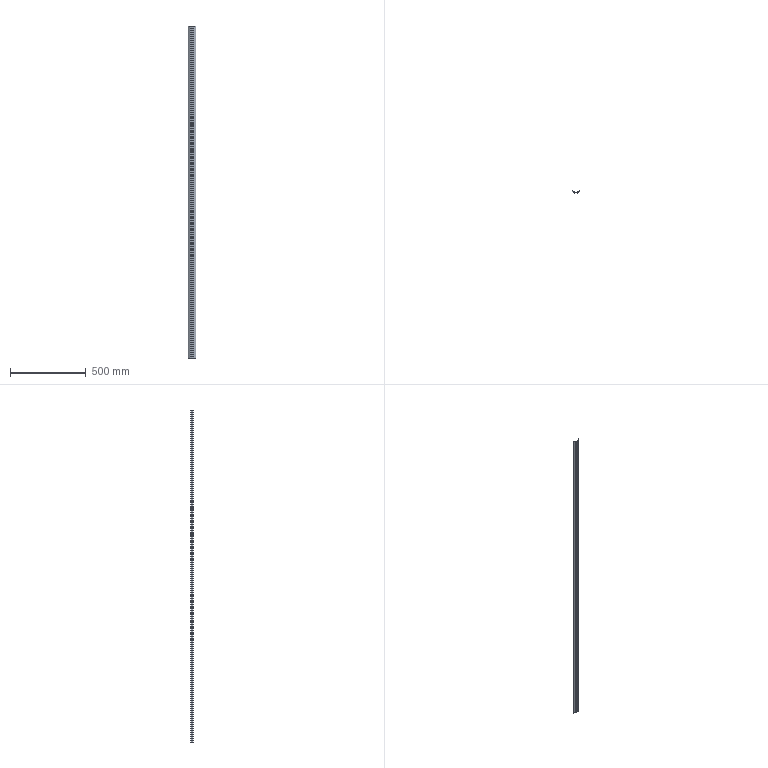Part | 1 solid | 32 faces | box 46.782 x 13.535 x 2190 mm | volume 175881 mm3 | plane 25 | cylinder 7 | commonest cylinder face diameters 67.994 x4 0.2 x2 65.594 x1
STEP:
#1=CARTESIAN_POINT('',(-11.25,9.786,-1095.));
#2=VERTEX_POINT('',#1);
#3=CARTESIAN_POINT('',(-11.25,5.783,-1095.));
#4=VERTEX_POINT('',#3);
#5=CARTESIAN_POINT('',(-11.25,9.786,-1095.));
#6=DIRECTION('',(0.,-1.,0.));
#7=VECTOR('',#6,1000.);
#8=LINE('',#5,#7);
#9=EDGE_CURVE('',#2,#4,#8,.T.);
#10=ORIENTED_EDGE('',*,*,#9,.T.);
#11=CARTESIAN_POINT('',(-11.25,5.783,1095.));
#12=VERTEX_POINT('',#11);
#13=CARTESIAN_POINT('',(-11.25,5.783,1095.));
#14=DIRECTION('',(0.,0.,-1.));
#15=VECTOR('',#14,1000.);
#16=LINE('',#13,#15);
#17=EDGE_CURVE('',#12,#4,#16,.T.);
#18=ORIENTED_EDGE('',*,*,#17,.F.);
#19=CARTESIAN_POINT('',(-11.25,9.786,1095.));
#20=VERTEX_POINT('',#19);
#21=CARTESIAN_POINT('',(-11.25,9.786,1095.));
#22=DIRECTION('',(0.,-1.,0.));
#23=VECTOR('',#22,1000.);
#24=LINE('',#21,#23);
#25=EDGE_CURVE('',#20,#12,#24,.T.);
#26=ORIENTED_EDGE('',*,*,#25,.F.);
#27=CARTESIAN_POINT('',(-11.25,9.786,1095.));
#28=DIRECTION('',(0.,0.,-1.));
#29=VECTOR('',#28,1000.);
#30=LINE('',#27,#29);
#31=EDGE_CURVE('',#20,#2,#30,.T.);
#32=ORIENTED_EDGE('',*,*,#31,.T.);
#33=EDGE_LOOP('',(#10,#18,#26,#32));
#34=FACE_OUTER_BOUND('',#33,.T.);
#35=CARTESIAN_POINT('',(-11.25,9.786,1095.));
#36=DIRECTION('',(1.,0.,0.));
#37=DIRECTION('',(0.,0.,-1.));
#38=AXIS2_PLACEMENT_3D('',#35,#36,#37);
#39=PLANE('',#38);
#40=ADVANCED_FACE('',(#34),#39,.F.);
#41=CARTESIAN_POINT('',(-10.667,5.2,-1095.));
#42=VERTEX_POINT('',#41);
#43=CARTESIAN_POINT('',(-11.25,5.783,-1095.));
#44=DIRECTION('',(0.7071,-0.7071,0.));
#45=VECTOR('',#44,1000.);
#46=LINE('',#43,#45);
#47=EDGE_CURVE('',#4,#42,#46,.T.);
#48=ORIENTED_EDGE('',*,*,#47,.T.);
#49=CARTESIAN_POINT('',(-10.667,5.2,1095.));
#50=VERTEX_POINT('',#49);
#51=CARTESIAN_POINT('',(-10.667,5.2,1095.));
#52=DIRECTION('',(0.,0.,-1.));
#53=VECTOR('',#52,1000.);
#54=LINE('',#51,#53);
#55=EDGE_CURVE('',#50,#42,#54,.T.);
#56=ORIENTED_EDGE('',*,*,#55,.F.);
#57=CARTESIAN_POINT('',(-11.25,5.783,1095.));
#58=DIRECTION('',(0.7071,-0.7071,0.));
#59=VECTOR('',#58,1000.);
#60=LINE('',#57,#59);
#61=EDGE_CURVE('',#12,#50,#60,.T.);
#62=ORIENTED_EDGE('',*,*,#61,.F.);
#63=ORIENTED_EDGE('',*,*,#17,.T.);
#64=EDGE_LOOP('',(#48,#56,#62,#63));
#65=FACE_OUTER_BOUND('',#64,.T.);
#66=CARTESIAN_POINT('',(-11.25,5.783,1095.));
#67=DIRECTION('',(0.7071,0.7071,0.));
#68=DIRECTION('',(-0.7071,0.7071,0.));
#69=AXIS2_PLACEMENT_3D('',#66,#67,#68);
#70=PLANE('',#69);
#71=ADVANCED_FACE('',(#65),#70,.F.);
#72=CARTESIAN_POINT('',(-8.25,5.2,-1095.));
#73=VERTEX_POINT('',#72);
#74=CARTESIAN_POINT('',(-10.667,5.2,-1095.));
#75=DIRECTION('',(1.,0.,0.));
#76=VECTOR('',#75,1000.);
#77=LINE('',#74,#76);
#78=EDGE_CURVE('',#42,#73,#77,.T.);
#79=ORIENTED_EDGE('',*,*,#78,.T.);
#80=CARTESIAN_POINT('',(-8.25,5.2,1095.));
#81=VERTEX_POINT('',#80);
#82=CARTESIAN_POINT('',(-8.25,5.2,1095.));
#83=DIRECTION('',(0.,0.,-1.));
#84=VECTOR('',#83,1000.);
#85=LINE('',#82,#84);
#86=EDGE_CURVE('',#81,#73,#85,.T.);
#87=ORIENTED_EDGE('',*,*,#86,.F.);
#88=CARTESIAN_POINT('',(-10.667,5.2,1095.));
#89=DIRECTION('',(1.,0.,0.));
#90=VECTOR('',#89,1000.);
#91=LINE('',#88,#90);
#92=EDGE_CURVE('',#50,#81,#91,.T.);
#93=ORIENTED_EDGE('',*,*,#92,.F.);
#94=ORIENTED_EDGE('',*,*,#55,.T.);
#95=EDGE_LOOP('',(#79,#87,#93,#94));
#96=FACE_OUTER_BOUND('',#95,.T.);
#97=CARTESIAN_POINT('',(-10.667,5.2,1095.));
#98=DIRECTION('',(0.,1.,0.));
#99=DIRECTION('',(0.,0.,1.));
#100=AXIS2_PLACEMENT_3D('',#97,#98,#99);
#101=PLANE('',#100);
#102=ADVANCED_FACE('',(#96),#101,.F.);
#103=CARTESIAN_POINT('',(-8.25,6.,-1095.));
#104=VERTEX_POINT('',#103);
#105=CARTESIAN_POINT('',(-8.25,5.2,-1095.));
#106=DIRECTION('',(0.,1.,0.));
#107=VECTOR('',#106,1000.);
#108=LINE('',#105,#107);
#109=EDGE_CURVE('',#73,#104,#108,.T.);
#110=ORIENTED_EDGE('',*,*,#109,.T.);
#111=CARTESIAN_POINT('',(-8.25,6.,1095.));
#112=VERTEX_POINT('',#111);
#113=CARTESIAN_POINT('',(-8.25,6.,1095.));
#114=DIRECTION('',(0.,0.,-1.));
#115=VECTOR('',#114,1000.);
#116=LINE('',#113,#115);
#117=EDGE_CURVE('',#112,#104,#116,.T.);
#118=ORIENTED_EDGE('',*,*,#117,.F.);
#119=CARTESIAN_POINT('',(-8.25,5.2,1095.));
#120=DIRECTION('',(0.,1.,0.));
#121=VECTOR('',#120,1000.);
#122=LINE('',#119,#121);
#123=EDGE_CURVE('',#81,#112,#122,.T.);
#124=ORIENTED_EDGE('',*,*,#123,.F.);
#125=ORIENTED_EDGE('',*,*,#86,.T.);
#126=EDGE_LOOP('',(#110,#118,#124,#125));
#127=FACE_OUTER_BOUND('',#126,.T.);
#128=CARTESIAN_POINT('',(-8.25,5.2,1095.));
#129=DIRECTION('',(-1.,0.,0.));
#130=DIRECTION('',(0.,0.,1.));
#131=AXIS2_PLACEMENT_3D('',#128,#129,#130);
#132=PLANE('',#131);
#133=ADVANCED_FACE('',(#127),#132,.F.);
#134=CARTESIAN_POINT('',(-10.25,6.,-1095.));
#135=VERTEX_POINT('',#134);
#136=CARTESIAN_POINT('',(-8.25,6.,-1095.));
#137=DIRECTION('',(-1.,0.,0.));
#138=VECTOR('',#137,1000.);
#139=LINE('',#136,#138);
#140=EDGE_CURVE('',#104,#135,#139,.T.);
#141=ORIENTED_EDGE('',*,*,#140,.T.);
#142=CARTESIAN_POINT('',(-10.25,6.,1095.));
#143=VERTEX_POINT('',#142);
#144=CARTESIAN_POINT('',(-10.25,6.,1095.));
#145=DIRECTION('',(0.,0.,-1.));
#146=VECTOR('',#145,1000.);
#147=LINE('',#144,#146);
#148=EDGE_CURVE('',#143,#135,#147,.T.);
#149=ORIENTED_EDGE('',*,*,#148,.F.);
#150=CARTESIAN_POINT('',(-8.25,6.,1095.));
#151=DIRECTION('',(-1.,0.,0.));
#152=VECTOR('',#151,1000.);
#153=LINE('',#150,#152);
#154=EDGE_CURVE('',#112,#143,#153,.T.);
#155=ORIENTED_EDGE('',*,*,#154,.F.);
#156=ORIENTED_EDGE('',*,*,#117,.T.);
#157=EDGE_LOOP('',(#141,#149,#155,#156));
#158=FACE_OUTER_BOUND('',#157,.T.);
#159=CARTESIAN_POINT('',(-8.25,6.,1095.));
#160=DIRECTION('',(0.,-1.,0.));
#161=DIRECTION('',(0.,0.,-1.));
#162=AXIS2_PLACEMENT_3D('',#159,#160,#161);
#163=PLANE('',#162);
#164=ADVANCED_FACE('',(#158),#163,.F.);
#165=CARTESIAN_POINT('',(-10.25,7.726,-1095.));
#166=VERTEX_POINT('',#165);
#167=CARTESIAN_POINT('',(-10.25,6.,-1095.));
#168=DIRECTION('',(0.,1.,0.));
#169=VECTOR('',#168,1000.);
#170=LINE('',#167,#169);
#171=EDGE_CURVE('',#135,#166,#170,.T.);
#172=ORIENTED_EDGE('',*,*,#171,.T.);
#173=CARTESIAN_POINT('',(-10.25,7.726,1095.));
#174=VERTEX_POINT('',#173);
#175=CARTESIAN_POINT('',(-10.25,7.726,1095.));
#176=DIRECTION('',(0.,0.,-1.));
#177=VECTOR('',#176,1000.);
#178=LINE('',#175,#177);
#179=EDGE_CURVE('',#174,#166,#178,.T.);
#180=ORIENTED_EDGE('',*,*,#179,.F.);
#181=CARTESIAN_POINT('',(-10.25,6.,1095.));
#182=DIRECTION('',(0.,1.,0.));
#183=VECTOR('',#182,1000.);
#184=LINE('',#181,#183);
#185=EDGE_CURVE('',#143,#174,#184,.T.);
#186=ORIENTED_EDGE('',*,*,#185,.F.);
#187=ORIENTED_EDGE('',*,*,#148,.T.);
#188=EDGE_LOOP('',(#172,#180,#186,#187));
#189=FACE_OUTER_BOUND('',#188,.T.);
#190=CARTESIAN_POINT('',(-10.25,6.,1095.));
#191=DIRECTION('',(-1.,0.,0.));
#192=DIRECTION('',(0.,0.,1.));
#193=AXIS2_PLACEMENT_3D('',#190,#191,#192);
#194=PLANE('',#193);
#195=ADVANCED_FACE('',(#189),#194,.F.);
#196=CARTESIAN_POINT('',(-9.,7.725,-1095.));
#197=VERTEX_POINT('',#196);
#198=CARTESIAN_POINT('',(-10.25,7.726,-1095.));
#199=DIRECTION('',(1.,-0.001291,0.));
#200=VECTOR('',#199,1000.);
#201=LINE('',#198,#200);
#202=EDGE_CURVE('',#166,#197,#201,.T.);
#203=ORIENTED_EDGE('',*,*,#202,.T.);
#204=CARTESIAN_POINT('',(-9.,7.725,1095.));
#205=VERTEX_POINT('',#204);
#206=CARTESIAN_POINT('',(-9.,7.725,1095.));
#207=DIRECTION('',(0.,0.,-1.));
#208=VECTOR('',#207,1000.);
#209=LINE('',#206,#208);
#210=EDGE_CURVE('',#205,#197,#209,.T.);
#211=ORIENTED_EDGE('',*,*,#210,.F.);
#212=CARTESIAN_POINT('',(-10.25,7.726,1095.));
#213=DIRECTION('',(1.,-0.001291,0.));
#214=VECTOR('',#213,1000.);
#215=LINE('',#212,#214);
#216=EDGE_CURVE('',#174,#205,#215,.T.);
#217=ORIENTED_EDGE('',*,*,#216,.F.);
#218=ORIENTED_EDGE('',*,*,#179,.T.);
#219=EDGE_LOOP('',(#203,#211,#217,#218));
#220=FACE_OUTER_BOUND('',#219,.T.);
#221=CARTESIAN_POINT('',(-10.25,7.726,1095.));
#222=DIRECTION('',(0.001291,1.,0.));
#223=DIRECTION('',(-1.,0.001291,0.));
#224=AXIS2_PLACEMENT_3D('',#221,#222,#223);
#225=PLANE('',#224);
#226=ADVANCED_FACE('',(#220),#225,.F.);
#227=CARTESIAN_POINT('',(-8.25,8.474,-1095.));
#228=VERTEX_POINT('',#227);
#229=CARTESIAN_POINT('',(-9.,7.725,-1095.));
#230=DIRECTION('',(0.7076,0.7067,0.));
#231=VECTOR('',#230,1000.);
#232=LINE('',#229,#231);
#233=EDGE_CURVE('',#197,#228,#232,.T.);
#234=ORIENTED_EDGE('',*,*,#233,.T.);
#235=CARTESIAN_POINT('',(-8.25,8.474,1095.));
#236=VERTEX_POINT('',#235);
#237=CARTESIAN_POINT('',(-8.25,8.474,1095.));
#238=DIRECTION('',(0.,0.,-1.));
#239=VECTOR('',#238,1000.);
#240=LINE('',#237,#239);
#241=EDGE_CURVE('',#236,#228,#240,.T.);
#242=ORIENTED_EDGE('',*,*,#241,.F.);
#243=CARTESIAN_POINT('',(-9.,7.725,1095.));
#244=DIRECTION('',(0.7076,0.7067,0.));
#245=VECTOR('',#244,1000.);
#246=LINE('',#243,#245);
#247=EDGE_CURVE('',#205,#236,#246,.T.);
#248=ORIENTED_EDGE('',*,*,#247,.F.);
#249=ORIENTED_EDGE('',*,*,#210,.T.);
#250=EDGE_LOOP('',(#234,#242,#248,#249));
#251=FACE_OUTER_BOUND('',#250,.T.);
#252=CARTESIAN_POINT('',(-9.,7.725,1095.));
#253=DIRECTION('',(-0.7067,0.7076,0.));
#254=DIRECTION('',(-0.7076,-0.7067,0.));
#255=AXIS2_PLACEMENT_3D('',#252,#253,#254);
#256=PLANE('',#255);
#257=ADVANCED_FACE('',(#251),#256,.F.);
#258=CARTESIAN_POINT('',(-8.25,8.887,-1095.));
#259=VERTEX_POINT('',#258);
#260=CARTESIAN_POINT('',(-8.25,8.474,-1095.));
#261=DIRECTION('',(0.,1.,0.));
#262=VECTOR('',#261,1000.);
#263=LINE('',#260,#262);
#264=EDGE_CURVE('',#228,#259,#263,.T.);
#265=ORIENTED_EDGE('',*,*,#264,.T.);
#266=CARTESIAN_POINT('',(-8.25,8.887,1095.));
#267=VERTEX_POINT('',#266);
#268=CARTESIAN_POINT('',(-8.25,8.887,1095.));
#269=DIRECTION('',(0.,0.,-1.));
#270=VECTOR('',#269,1000.);
#271=LINE('',#268,#270);
#272=EDGE_CURVE('',#267,#259,#271,.T.);
#273=ORIENTED_EDGE('',*,*,#272,.F.);
#274=CARTESIAN_POINT('',(-8.25,8.474,1095.));
#275=DIRECTION('',(0.,1.,0.));
#276=VECTOR('',#275,1000.);
#277=LINE('',#274,#276);
#278=EDGE_CURVE('',#236,#267,#277,.T.);
#279=ORIENTED_EDGE('',*,*,#278,.F.);
#280=ORIENTED_EDGE('',*,*,#241,.T.);
#281=EDGE_LOOP('',(#265,#273,#279,#280));
#282=FACE_OUTER_BOUND('',#281,.T.);
#283=CARTESIAN_POINT('',(-8.25,8.474,1095.));
#284=DIRECTION('',(-1.,0.,0.));
#285=DIRECTION('',(0.,0.,1.));
#286=AXIS2_PLACEMENT_3D('',#283,#284,#285);
#287=PLANE('',#286);
#288=ADVANCED_FACE('',(#282),#287,.F.);
#289=CARTESIAN_POINT('',(-3.,8.003,-1095.));
#290=VERTEX_POINT('',#289);
#291=CARTESIAN_POINT('',(0.,41.867,-1095.));
#292=DIRECTION('',(0.,0.,1.));
#293=DIRECTION('',(1.,0.,0.));
#294=AXIS2_PLACEMENT_3D('',#291,#292,#293);
#295=CIRCLE('',#294,33.997);
#296=EDGE_CURVE('',#259,#290,#295,.T.);
#297=ORIENTED_EDGE('',*,*,#296,.T.);
#298=CARTESIAN_POINT('',(-3.,8.003,1095.));
#299=VERTEX_POINT('',#298);
#300=CARTESIAN_POINT('',(-3.,8.003,1095.));
#301=DIRECTION('',(0.,0.,-1.));
#302=VECTOR('',#301,1000.);
#303=LINE('',#300,#302);
#304=EDGE_CURVE('',#299,#290,#303,.T.);
#305=ORIENTED_EDGE('',*,*,#304,.F.);
#306=CARTESIAN_POINT('',(0.,41.867,1095.));
#307=DIRECTION('',(0.,0.,1.));
#308=DIRECTION('',(1.,0.,0.));
#309=AXIS2_PLACEMENT_3D('',#306,#307,#308);
#310=CIRCLE('',#309,33.997);
#311=EDGE_CURVE('',#267,#299,#310,.T.);
#312=ORIENTED_EDGE('',*,*,#311,.F.);
#313=ORIENTED_EDGE('',*,*,#272,.T.);
#314=EDGE_LOOP('',(#297,#305,#312,#313));
#315=FACE_OUTER_BOUND('',#314,.T.);
#316=CARTESIAN_POINT('',(0.,41.867,1095.));
#317=DIRECTION('',(0.,0.,-1.));
#318=DIRECTION('',(-1.,0.,0.));
#319=AXIS2_PLACEMENT_3D('',#316,#317,#318);
#320=CYLINDRICAL_SURFACE('',#319,33.997);
#321=ADVANCED_FACE('',(#315),#320,.T.);
#322=CARTESIAN_POINT('',(-3.,7.702,-1095.));
#323=VERTEX_POINT('',#322);
#324=CARTESIAN_POINT('',(-3.,8.003,-1095.));
#325=DIRECTION('',(0.,-1.,0.));
#326=VECTOR('',#325,1000.);
#327=LINE('',#324,#326);
#328=EDGE_CURVE('',#290,#323,#327,.T.);
#329=ORIENTED_EDGE('',*,*,#328,.T.);
#330=CARTESIAN_POINT('',(-3.,7.702,1095.));
#331=VERTEX_POINT('',#330);
#332=CARTESIAN_POINT('',(-3.,7.702,1095.));
#333=DIRECTION('',(0.,0.,-1.));
#334=VECTOR('',#333,1000.);
#335=LINE('',#332,#334);
#336=EDGE_CURVE('',#331,#323,#335,.T.);
#337=ORIENTED_EDGE('',*,*,#336,.F.);
#338=CARTESIAN_POINT('',(-3.,8.003,1095.));
#339=DIRECTION('',(0.,-1.,0.));
#340=VECTOR('',#339,1000.);
#341=LINE('',#338,#340);
#342=EDGE_CURVE('',#299,#331,#341,.T.);
#343=ORIENTED_EDGE('',*,*,#342,.F.);
#344=ORIENTED_EDGE('',*,*,#304,.T.);
#345=EDGE_LOOP('',(#329,#337,#343,#344));
#346=FACE_OUTER_BOUND('',#345,.T.);
#347=CARTESIAN_POINT('',(-3.,8.003,1095.));
#348=DIRECTION('',(1.,0.,0.));
#349=DIRECTION('',(0.,0.,-1.));
#350=AXIS2_PLACEMENT_3D('',#347,#348,#349);
#351=PLANE('',#350);
#352=ADVANCED_FACE('',(#346),#351,.F.);
#353=CARTESIAN_POINT('',(3.,7.702,-1095.));
#354=VERTEX_POINT('',#353);
#355=CARTESIAN_POINT('',(-3.,7.702,-1095.));
#356=DIRECTION('',(1.,0.,0.));
#357=VECTOR('',#356,1000.);
#358=LINE('',#355,#357);
#359=EDGE_CURVE('',#323,#354,#358,.T.);
#360=ORIENTED_EDGE('',*,*,#359,.T.);
#361=CARTESIAN_POINT('',(3.,7.702,1095.));
#362=VERTEX_POINT('',#361);
#363=CARTESIAN_POINT('',(3.,7.702,1095.));
#364=DIRECTION('',(0.,0.,-1.));
#365=VECTOR('',#364,1000.);
#366=LINE('',#363,#365);
#367=EDGE_CURVE('',#362,#354,#366,.T.);
#368=ORIENTED_EDGE('',*,*,#367,.F.);
#369=CARTESIAN_POINT('',(-3.,7.702,1095.));
#370=DIRECTION('',(1.,0.,0.));
#371=VECTOR('',#370,1000.);
#372=LINE('',#369,#371);
#373=EDGE_CURVE('',#331,#362,#372,.T.);
#374=ORIENTED_EDGE('',*,*,#373,.F.);
#375=ORIENTED_EDGE('',*,*,#336,.T.);
#376=EDGE_LOOP('',(#360,#368,#374,#375));
#377=FACE_OUTER_BOUND('',#376,.T.);
#378=CARTESIAN_POINT('',(-3.,7.702,1095.));
#379=DIRECTION('',(0.,1.,0.));
#380=DIRECTION('',(0.,0.,1.));
#381=AXIS2_PLACEMENT_3D('',#378,#379,#380);
#382=PLANE('',#381);
#383=ADVANCED_FACE('',(#377),#382,.F.);
#384=CARTESIAN_POINT('',(3.,8.003,-1095.));
#385=VERTEX_POINT('',#384);
#386=CARTESIAN_POINT('',(3.,7.702,-1095.));
#387=DIRECTION('',(0.,1.,0.));
#388=VECTOR('',#387,1000.);
#389=LINE('',#386,#388);
#390=EDGE_CURVE('',#354,#385,#389,.T.);
#391=ORIENTED_EDGE('',*,*,#390,.T.);
#392=CARTESIAN_POINT('',(3.,8.003,1095.));
#393=VERTEX_POINT('',#392);
#394=CARTESIAN_POINT('',(3.,8.003,1095.));
#395=DIRECTION('',(0.,0.,-1.));
#396=VECTOR('',#395,1000.);
#397=LINE('',#394,#396);
#398=EDGE_CURVE('',#393,#385,#397,.T.);
#399=ORIENTED_EDGE('',*,*,#398,.F.);
#400=CARTESIAN_POINT('',(3.,7.702,1095.));
#401=DIRECTION('',(0.,1.,0.));
#402=VECTOR('',#401,1000.);
#403=LINE('',#400,#402);
#404=EDGE_CURVE('',#362,#393,#403,.T.);
#405=ORIENTED_EDGE('',*,*,#404,.F.);
#406=ORIENTED_EDGE('',*,*,#367,.T.);
#407=EDGE_LOOP('',(#391,#399,#405,#406));
#408=FACE_OUTER_BOUND('',#407,.T.);
#409=CARTESIAN_POINT('',(3.,7.702,1095.));
#410=DIRECTION('',(-1.,0.,0.));
#411=DIRECTION('',(0.,0.,1.));
#412=AXIS2_PLACEMENT_3D('',#409,#410,#411);
#413=PLANE('',#412);
#414=ADVANCED_FACE('',(#408),#413,.F.);
#415=CARTESIAN_POINT('',(8.25,8.887,-1095.));
#416=VERTEX_POINT('',#415);
#417=CARTESIAN_POINT('',(0.,41.867,-1095.));
#418=DIRECTION('',(0.,0.,1.));
#419=DIRECTION('',(1.,0.,0.));
#420=AXIS2_PLACEMENT_3D('',#417,#418,#419);
#421=CIRCLE('',#420,33.997);
#422=EDGE_CURVE('',#385,#416,#421,.T.);
#423=ORIENTED_EDGE('',*,*,#422,.T.);
#424=CARTESIAN_POINT('',(8.25,8.887,1095.));
#425=VERTEX_POINT('',#424);
#426=CARTESIAN_POINT('',(8.25,8.887,1095.));
#427=DIRECTION('',(0.,0.,-1.));
#428=VECTOR('',#427,1000.);
#429=LINE('',#426,#428);
#430=EDGE_CURVE('',#425,#416,#429,.T.);
#431=ORIENTED_EDGE('',*,*,#430,.F.);
#432=CARTESIAN_POINT('',(0.,41.867,1095.));
#433=DIRECTION('',(0.,0.,1.));
#434=DIRECTION('',(1.,0.,0.));
#435=AXIS2_PLACEMENT_3D('',#432,#433,#434);
#436=CIRCLE('',#435,33.997);
#437=EDGE_CURVE('',#393,#425,#436,.T.);
#438=ORIENTED_EDGE('',*,*,#437,.F.);
#439=ORIENTED_EDGE('',*,*,#398,.T.);
#440=EDGE_LOOP('',(#423,#431,#438,#439));
#441=FACE_OUTER_BOUND('',#440,.T.);
#442=CARTESIAN_POINT('',(0.,41.867,1095.));
#443=DIRECTION('',(0.,0.,-1.));
#444=DIRECTION('',(-1.,0.,0.));
#445=AXIS2_PLACEMENT_3D('',#442,#443,#444);
#446=CYLINDRICAL_SURFACE('',#445,33.997);
#447=ADVANCED_FACE('',(#441),#446,.T.);
#448=CARTESIAN_POINT('',(8.25,8.474,-1095.));
#449=VERTEX_POINT('',#448);
#450=CARTESIAN_POINT('',(8.25,8.887,-1095.));
#451=DIRECTION('',(0.,-1.,0.));
#452=VECTOR('',#451,1000.);
#453=LINE('',#450,#452);
#454=EDGE_CURVE('',#416,#449,#453,.T.);
#455=ORIENTED_EDGE('',*,*,#454,.T.);
#456=CARTESIAN_POINT('',(8.25,8.474,1095.));
#457=VERTEX_POINT('',#456);
#458=CARTESIAN_POINT('',(8.25,8.474,1095.));
#459=DIRECTION('',(0.,0.,-1.));
#460=VECTOR('',#459,1000.);
#461=LINE('',#458,#460);
#462=EDGE_CURVE('',#457,#449,#461,.T.);
#463=ORIENTED_EDGE('',*,*,#462,.F.);
#464=CARTESIAN_POINT('',(8.25,8.887,1095.));
#465=DIRECTION('',(0.,-1.,0.));
#466=VECTOR('',#465,1000.);
#467=LINE('',#464,#466);
#468=EDGE_CURVE('',#425,#457,#467,.T.);
#469=ORIENTED_EDGE('',*,*,#468,.F.);
#470=ORIENTED_EDGE('',*,*,#430,.T.);
#471=EDGE_LOOP('',(#455,#463,#469,#470));
#472=FACE_OUTER_BOUND('',#471,.T.);
#473=CARTESIAN_POINT('',(8.25,8.887,1095.));
#474=DIRECTION('',(1.,0.,0.));
#475=DIRECTION('',(0.,0.,-1.));
#476=AXIS2_PLACEMENT_3D('',#473,#474,#475);
#477=PLANE('',#476);
#478=ADVANCED_FACE('',(#472),#477,.F.);
#479=CARTESIAN_POINT('',(9.,7.725,-1095.));
#480=VERTEX_POINT('',#479);
#481=CARTESIAN_POINT('',(8.25,8.474,-1095.));
#482=DIRECTION('',(0.7076,-0.7067,0.));
#483=VECTOR('',#482,1000.);
#484=LINE('',#481,#483);
#485=EDGE_CURVE('',#449,#480,#484,.T.);
#486=ORIENTED_EDGE('',*,*,#485,.T.);
#487=CARTESIAN_POINT('',(9.,7.725,1095.));
#488=VERTEX_POINT('',#487);
#489=CARTESIAN_POINT('',(9.,7.725,1095.));
#490=DIRECTION('',(0.,0.,-1.));
#491=VECTOR('',#490,1000.);
#492=LINE('',#489,#491);
#493=EDGE_CURVE('',#488,#480,#492,.T.);
#494=ORIENTED_EDGE('',*,*,#493,.F.);
#495=CARTESIAN_POINT('',(8.25,8.474,1095.));
#496=DIRECTION('',(0.7076,-0.7067,0.));
#497=VECTOR('',#496,1000.);
#498=LINE('',#495,#497);
#499=EDGE_CURVE('',#457,#488,#498,.T.);
#500=ORIENTED_EDGE('',*,*,#499,.F.);
#501=ORIENTED_EDGE('',*,*,#462,.T.);
#502=EDGE_LOOP('',(#486,#494,#500,#501));
#503=FACE_OUTER_BOUND('',#502,.T.);
#504=CARTESIAN_POINT('',(8.25,8.474,1095.));
#505=DIRECTION('',(0.7067,0.7076,0.));
#506=DIRECTION('',(-0.7076,0.7067,0.));
#507=AXIS2_PLACEMENT_3D('',#504,#505,#506);
#508=PLANE('',#507);
#509=ADVANCED_FACE('',(#503),#508,.F.);
#510=CARTESIAN_POINT('',(10.25,7.726,-1095.));
#511=VERTEX_POINT('',#510);
#512=CARTESIAN_POINT('',(9.,7.725,-1095.));
#513=DIRECTION('',(1.,0.001291,0.));
#514=VECTOR('',#513,1000.);
#515=LINE('',#512,#514);
#516=EDGE_CURVE('',#480,#511,#515,.T.);
#517=ORIENTED_EDGE('',*,*,#516,.T.);
#518=CARTESIAN_POINT('',(10.25,7.726,1095.));
#519=VERTEX_POINT('',#518);
#520=CARTESIAN_POINT('',(10.25,7.726,1095.));
#521=DIRECTION('',(0.,0.,-1.));
#522=VECTOR('',#521,1000.);
#523=LINE('',#520,#522);
#524=EDGE_CURVE('',#519,#511,#523,.T.);
#525=ORIENTED_EDGE('',*,*,#524,.F.);
#526=CARTESIAN_POINT('',(9.,7.725,1095.));
#527=DIRECTION('',(1.,0.001291,0.));
#528=VECTOR('',#527,1000.);
#529=LINE('',#526,#528);
#530=EDGE_CURVE('',#488,#519,#529,.T.);
#531=ORIENTED_EDGE('',*,*,#530,.F.);
#532=ORIENTED_EDGE('',*,*,#493,.T.);
#533=EDGE_LOOP('',(#517,#525,#531,#532));
#534=FACE_OUTER_BOUND('',#533,.T.);
#535=CARTESIAN_POINT('',(9.,7.725,1095.));
#536=DIRECTION('',(-0.001291,1.,0.));
#537=DIRECTION('',(-1.,-0.001291,0.));
#538=AXIS2_PLACEMENT_3D('',#535,#536,#537);
#539=PLANE('',#538);
#540=ADVANCED_FACE('',(#534),#539,.F.);
#541=CARTESIAN_POINT('',(10.25,6.,-1095.));
#542=VERTEX_POINT('',#541);
#543=CARTESIAN_POINT('',(10.25,7.726,-1095.));
#544=DIRECTION('',(0.,-1.,0.));
#545=VECTOR('',#544,1000.);
#546=LINE('',#543,#545);
#547=EDGE_CURVE('',#511,#542,#546,.T.);
#548=ORIENTED_EDGE('',*,*,#547,.T.);
#549=CARTESIAN_POINT('',(10.25,6.,1095.));
#550=VERTEX_POINT('',#549);
#551=CARTESIAN_POINT('',(10.25,6.,1095.));
#552=DIRECTION('',(0.,0.,-1.));
#553=VECTOR('',#552,1000.);
#554=LINE('',#551,#553);
#555=EDGE_CURVE('',#550,#542,#554,.T.);
#556=ORIENTED_EDGE('',*,*,#555,.F.);
#557=CARTESIAN_POINT('',(10.25,7.726,1095.));
#558=DIRECTION('',(0.,-1.,0.));
#559=VECTOR('',#558,1000.);
#560=LINE('',#557,#559);
#561=EDGE_CURVE('',#519,#550,#560,.T.);
#562=ORIENTED_EDGE('',*,*,#561,.F.);
#563=ORIENTED_EDGE('',*,*,#524,.T.);
#564=EDGE_LOOP('',(#548,#556,#562,#563));
#565=FACE_OUTER_BOUND('',#564,.T.);
#566=CARTESIAN_POINT('',(10.25,7.726,1095.));
#567=DIRECTION('',(1.,0.,0.));
#568=DIRECTION('',(0.,0.,-1.));
#569=AXIS2_PLACEMENT_3D('',#566,#567,#568);
#570=PLANE('',#569);
#571=ADVANCED_FACE('',(#565),#570,.F.);
#572=CARTESIAN_POINT('',(8.25,6.,-1095.));
#573=VERTEX_POINT('',#572);
#574=CARTESIAN_POINT('',(10.25,6.,-1095.));
#575=DIRECTION('',(-1.,0.,0.));
#576=VECTOR('',#575,1000.);
#577=LINE('',#574,#576);
#578=EDGE_CURVE('',#542,#573,#577,.T.);
#579=ORIENTED_EDGE('',*,*,#578,.T.);
#580=CARTESIAN_POINT('',(8.25,6.,1095.));
#581=VERTEX_POINT('',#580);
#582=CARTESIAN_POINT('',(8.25,6.,1095.));
#583=DIRECTION('',(0.,0.,-1.));
#584=VECTOR('',#583,1000.);
#585=LINE('',#582,#584);
#586=EDGE_CURVE('',#581,#573,#585,.T.);
#587=ORIENTED_EDGE('',*,*,#586,.F.);
#588=CARTESIAN_POINT('',(10.25,6.,1095.));
#589=DIRECTION('',(-1.,0.,0.));
#590=VECTOR('',#589,1000.);
#591=LINE('',#588,#590);
#592=EDGE_CURVE('',#550,#581,#591,.T.);
#593=ORIENTED_EDGE('',*,*,#592,.F.);
#594=ORIENTED_EDGE('',*,*,#555,.T.);
#595=EDGE_LOOP('',(#579,#587,#593,#594));
#596=FACE_OUTER_BOUND('',#595,.T.);
#597=CARTESIAN_POINT('',(10.25,6.,1095.));
#598=DIRECTION('',(0.,-1.,0.));
#599=DIRECTION('',(0.,0.,-1.));
#600=AXIS2_PLACEMENT_3D('',#597,#598,#599);
#601=PLANE('',#600);
#602=ADVANCED_FACE('',(#596),#601,.F.);
#603=CARTESIAN_POINT('',(8.25,5.2,-1095.));
#604=VERTEX_POINT('',#603);
#605=CARTESIAN_POINT('',(8.25,6.,-1095.));
#606=DIRECTION('',(0.,-1.,0.));
#607=VECTOR('',#606,1000.);
#608=LINE('',#605,#607);
#609=EDGE_CURVE('',#573,#604,#608,.T.);
#610=ORIENTED_EDGE('',*,*,#609,.T.);
#611=CARTESIAN_POINT('',(8.25,5.2,1095.));
#612=VERTEX_POINT('',#611);
#613=CARTESIAN_POINT('',(8.25,5.2,1095.));
#614=DIRECTION('',(0.,0.,-1.));
#615=VECTOR('',#614,1000.);
#616=LINE('',#613,#615);
#617=EDGE_CURVE('',#612,#604,#616,.T.);
#618=ORIENTED_EDGE('',*,*,#617,.F.);
#619=CARTESIAN_POINT('',(8.25,6.,1095.));
#620=DIRECTION('',(0.,-1.,0.));
#621=VECTOR('',#620,1000.);
#622=LINE('',#619,#621);
#623=EDGE_CURVE('',#581,#612,#622,.T.);
#624=ORIENTED_EDGE('',*,*,#623,.F.);
#625=ORIENTED_EDGE('',*,*,#586,.T.);
#626=EDGE_LOOP('',(#610,#618,#624,#625));
#627=FACE_OUTER_BOUND('',#626,.T.);
#628=CARTESIAN_POINT('',(8.25,6.,1095.));
#629=DIRECTION('',(1.,0.,0.));
#630=DIRECTION('',(0.,0.,-1.));
#631=AXIS2_PLACEMENT_3D('',#628,#629,#630);
#632=PLANE('',#631);
#633=ADVANCED_FACE('',(#627),#632,.F.);
#634=CARTESIAN_POINT('',(10.667,5.2,-1095.));
#635=VERTEX_POINT('',#634);
#636=CARTESIAN_POINT('',(8.25,5.2,-1095.));
#637=DIRECTION('',(1.,0.,0.));
#638=VECTOR('',#637,1000.);
#639=LINE('',#636,#638);
#640=EDGE_CURVE('',#604,#635,#639,.T.);
#641=ORIENTED_EDGE('',*,*,#640,.T.);
#642=CARTESIAN_POINT('',(10.667,5.2,1095.));
#643=VERTEX_POINT('',#642);
#644=CARTESIAN_POINT('',(10.667,5.2,1095.));
#645=DIRECTION('',(0.,0.,-1.));
#646=VECTOR('',#645,1000.);
#647=LINE('',#644,#646);
#648=EDGE_CURVE('',#643,#635,#647,.T.);
#649=ORIENTED_EDGE('',*,*,#648,.F.);
#650=CARTESIAN_POINT('',(8.25,5.2,1095.));
#651=DIRECTION('',(1.,0.,0.));
#652=VECTOR('',#651,1000.);
#653=LINE('',#650,#652);
#654=EDGE_CURVE('',#612,#643,#653,.T.);
#655=ORIENTED_EDGE('',*,*,#654,.F.);
#656=ORIENTED_EDGE('',*,*,#617,.T.);
#657=EDGE_LOOP('',(#641,#649,#655,#656));
#658=FACE_OUTER_BOUND('',#657,.T.);
#659=CARTESIAN_POINT('',(8.25,5.2,1095.));
#660=DIRECTION('',(0.,1.,0.));
#661=DIRECTION('',(0.,0.,1.));
#662=AXIS2_PLACEMENT_3D('',#659,#660,#661);
#663=PLANE('',#662);
#664=ADVANCED_FACE('',(#658),#663,.F.);
#665=CARTESIAN_POINT('',(11.25,5.783,-1095.));
#666=VERTEX_POINT('',#665);
#667=CARTESIAN_POINT('',(10.667,5.2,-1095.));
#668=DIRECTION('',(0.7071,0.7071,0.));
#669=VECTOR('',#668,1000.);
#670=LINE('',#667,#669);
#671=EDGE_CURVE('',#635,#666,#670,.T.);
#672=ORIENTED_EDGE('',*,*,#671,.T.);
#673=CARTESIAN_POINT('',(11.25,5.783,1095.));
#674=VERTEX_POINT('',#673);
#675=CARTESIAN_POINT('',(11.25,5.783,1095.));
#676=DIRECTION('',(0.,0.,-1.));
#677=VECTOR('',#676,1000.);
#678=LINE('',#675,#677);
#679=EDGE_CURVE('',#674,#666,#678,.T.);
#680=ORIENTED_EDGE('',*,*,#679,.F.);
#681=CARTESIAN_POINT('',(10.667,5.2,1095.));
#682=DIRECTION('',(0.7071,0.7071,0.));
#683=VECTOR('',#682,1000.);
#684=LINE('',#681,#683);
#685=EDGE_CURVE('',#643,#674,#684,.T.);
#686=ORIENTED_EDGE('',*,*,#685,.F.);
#687=ORIENTED_EDGE('',*,*,#648,.T.);
#688=EDGE_LOOP('',(#672,#680,#686,#687));
#689=FACE_OUTER_BOUND('',#688,.T.);
#690=CARTESIAN_POINT('',(10.667,5.2,1095.));
#691=DIRECTION('',(-0.7071,0.7071,0.));
#692=DIRECTION('',(-0.7071,-0.7071,0.));
#693=AXIS2_PLACEMENT_3D('',#690,#691,#692);
#694=PLANE('',#693);
#695=ADVANCED_FACE('',(#689),#694,.F.);
#696=CARTESIAN_POINT('',(11.25,9.786,-1095.));
#697=VERTEX_POINT('',#696);
#698=CARTESIAN_POINT('',(11.25,5.783,-1095.));
#699=DIRECTION('',(0.,1.,0.));
#700=VECTOR('',#699,1000.);
#701=LINE('',#698,#700);
#702=EDGE_CURVE('',#666,#697,#701,.T.);
#703=ORIENTED_EDGE('',*,*,#702,.T.);
#704=CARTESIAN_POINT('',(11.25,9.786,1095.));
#705=VERTEX_POINT('',#704);
#706=CARTESIAN_POINT('',(11.25,9.786,1095.));
#707=DIRECTION('',(0.,0.,-1.));
#708=VECTOR('',#707,1000.);
#709=LINE('',#706,#708);
#710=EDGE_CURVE('',#705,#697,#709,.T.);
#711=ORIENTED_EDGE('',*,*,#710,.F.);
#712=CARTESIAN_POINT('',(11.25,5.783,1095.));
#713=DIRECTION('',(0.,1.,0.));
#714=VECTOR('',#713,1000.);
#715=LINE('',#712,#714);
#716=EDGE_CURVE('',#674,#705,#715,.T.);
#717=ORIENTED_EDGE('',*,*,#716,.F.);
#718=ORIENTED_EDGE('',*,*,#679,.T.);
#719=EDGE_LOOP('',(#703,#711,#717,#718));
#720=FACE_OUTER_BOUND('',#719,.T.);
#721=CARTESIAN_POINT('',(11.25,5.783,1095.));
#722=DIRECTION('',(-1.,0.,0.));
#723=DIRECTION('',(0.,0.,1.));
#724=AXIS2_PLACEMENT_3D('',#721,#722,#723);
#725=PLANE('',#724);
#726=ADVANCED_FACE('',(#720),#725,.F.);
#727=CARTESIAN_POINT('',(23.391,17.196,-1095.));
#728=VERTEX_POINT('',#727);
#729=CARTESIAN_POINT('',(0.,41.867,-1095.));
#730=DIRECTION('',(0.,0.,1.));
#731=DIRECTION('',(1.,0.,0.));
#732=AXIS2_PLACEMENT_3D('',#729,#730,#731);
#733=CIRCLE('',#732,33.997);
#734=EDGE_CURVE('',#697,#728,#733,.T.);
#735=ORIENTED_EDGE('',*,*,#734,.T.);
#736=CARTESIAN_POINT('',(23.391,17.196,1095.));
#737=VERTEX_POINT('',#736);
#738=CARTESIAN_POINT('',(23.391,17.196,1095.));
#739=DIRECTION('',(0.,0.,-1.));
#740=VECTOR('',#739,1000.);
#741=LINE('',#738,#740);
#742=EDGE_CURVE('',#737,#728,#741,.T.);
#743=ORIENTED_EDGE('',*,*,#742,.F.);
#744=CARTESIAN_POINT('',(0.,41.867,1095.));
#745=DIRECTION('',(0.,0.,1.));
#746=DIRECTION('',(1.,0.,0.));
#747=AXIS2_PLACEMENT_3D('',#744,#745,#746);
#748=CIRCLE('',#747,33.997);
#749=EDGE_CURVE('',#705,#737,#748,.T.);
#750=ORIENTED_EDGE('',*,*,#749,.F.);
#751=ORIENTED_EDGE('',*,*,#710,.T.);
#752=EDGE_LOOP('',(#735,#743,#750,#751));
#753=FACE_OUTER_BOUND('',#752,.T.);
#754=CARTESIAN_POINT('',(0.,41.867,1095.));
#755=DIRECTION('',(0.,0.,-1.));
#756=DIRECTION('',(-1.,0.,0.));
#757=AXIS2_PLACEMENT_3D('',#754,#755,#756);
#758=CYLINDRICAL_SURFACE('',#757,33.997);
#759=ADVANCED_FACE('',(#753),#758,.T.);
#760=CARTESIAN_POINT('',(23.391,18.635,-1095.));
#761=VERTEX_POINT('',#760);
#762=CARTESIAN_POINT('',(23.391,17.196,-1095.));
#763=DIRECTION('',(0.,1.,0.));
#764=VECTOR('',#763,1000.);
#765=LINE('',#762,#764);
#766=EDGE_CURVE('',#728,#761,#765,.T.);
#767=ORIENTED_EDGE('',*,*,#766,.T.);
#768=CARTESIAN_POINT('',(23.391,18.635,1095.));
#769=VERTEX_POINT('',#768);
#770=CARTESIAN_POINT('',(23.391,18.635,1095.));
#771=DIRECTION('',(0.,0.,-1.));
#772=VECTOR('',#771,1000.);
#773=LINE('',#770,#772);
#774=EDGE_CURVE('',#769,#761,#773,.T.);
#775=ORIENTED_EDGE('',*,*,#774,.F.);
#776=CARTESIAN_POINT('',(23.391,17.196,1095.));
#777=DIRECTION('',(0.,1.,0.));
#778=VECTOR('',#777,1000.);
#779=LINE('',#776,#778);
#780=EDGE_CURVE('',#737,#769,#779,.T.);
#781=ORIENTED_EDGE('',*,*,#780,.F.);
#782=ORIENTED_EDGE('',*,*,#742,.T.);
#783=EDGE_LOOP('',(#767,#775,#781,#782));
#784=FACE_OUTER_BOUND('',#783,.T.);
#785=CARTESIAN_POINT('',(23.391,17.196,1095.));
#786=DIRECTION('',(-1.,0.,0.));
#787=DIRECTION('',(0.,0.,1.));
#788=AXIS2_PLACEMENT_3D('',#785,#786,#787);
#789=PLANE('',#788);
#790=ADVANCED_FACE('',(#784),#789,.F.);
#791=CARTESIAN_POINT('',(23.22,18.706,-1095.));
#792=VERTEX_POINT('',#791);
#793=CARTESIAN_POINT('',(23.291,18.635,-1095.));
#794=DIRECTION('',(0.,0.,1.));
#795=DIRECTION('',(1.,0.,0.));
#796=AXIS2_PLACEMENT_3D('',#793,#794,#795);
#797=CIRCLE('',#796,0.1);
#798=EDGE_CURVE('',#761,#792,#797,.T.);
#799=ORIENTED_EDGE('',*,*,#798,.T.);
#800=CARTESIAN_POINT('',(23.22,18.706,1095.));
#801=VERTEX_POINT('',#800);
#802=CARTESIAN_POINT('',(23.22,18.706,1095.));
#803=DIRECTION('',(0.,0.,-1.));
#804=VECTOR('',#803,1000.);
#805=LINE('',#802,#804);
#806=EDGE_CURVE('',#801,#792,#805,.T.);
#807=ORIENTED_EDGE('',*,*,#806,.F.);
#808=CARTESIAN_POINT('',(23.291,18.635,1095.));
#809=DIRECTION('',(0.,0.,1.));
#810=DIRECTION('',(1.,0.,0.));
#811=AXIS2_PLACEMENT_3D('',#808,#809,#810);
#812=CIRCLE('',#811,0.1);
#813=EDGE_CURVE('',#769,#801,#812,.T.);
#814=ORIENTED_EDGE('',*,*,#813,.F.);
#815=ORIENTED_EDGE('',*,*,#774,.T.);
#816=EDGE_LOOP('',(#799,#807,#814,#815));
#817=FACE_OUTER_BOUND('',#816,.T.);
#818=CARTESIAN_POINT('',(23.291,18.635,1095.));
#819=DIRECTION('',(0.,0.,-1.));
#820=DIRECTION('',(-1.,0.,0.));
#821=AXIS2_PLACEMENT_3D('',#818,#819,#820);
#822=CYLINDRICAL_SURFACE('',#821,0.1);
#823=ADVANCED_FACE('',(#817),#822,.T.);
#824=CARTESIAN_POINT('',(-23.22,18.706,-1095.));
#825=VERTEX_POINT('',#824);
#826=CARTESIAN_POINT('',(0.,41.867,-1095.));
#827=DIRECTION('',(0.,0.,-1.));
#828=DIRECTION('',(1.,0.,0.));
#829=AXIS2_PLACEMENT_3D('',#826,#827,#828);
#830=CIRCLE('',#829,32.797);
#831=EDGE_CURVE('',#792,#825,#830,.T.);
#832=ORIENTED_EDGE('',*,*,#831,.T.);
#833=CARTESIAN_POINT('',(-23.22,18.706,1095.));
#834=VERTEX_POINT('',#833);
#835=CARTESIAN_POINT('',(-23.22,18.706,1095.));
#836=DIRECTION('',(0.,0.,-1.));
#837=VECTOR('',#836,1000.);
#838=LINE('',#835,#837);
#839=EDGE_CURVE('',#834,#825,#838,.T.);
#840=ORIENTED_EDGE('',*,*,#839,.F.);
#841=CARTESIAN_POINT('',(0.,41.867,1095.));
#842=DIRECTION('',(0.,0.,-1.));
#843=DIRECTION('',(1.,0.,0.));
#844=AXIS2_PLACEMENT_3D('',#841,#842,#843);
#845=CIRCLE('',#844,32.797);
#846=EDGE_CURVE('',#801,#834,#845,.T.);
#847=ORIENTED_EDGE('',*,*,#846,.F.);
#848=ORIENTED_EDGE('',*,*,#806,.T.);
#849=EDGE_LOOP('',(#832,#840,#847,#848));
#850=FACE_OUTER_BOUND('',#849,.T.);
#851=CARTESIAN_POINT('',(0.,41.867,1095.));
#852=DIRECTION('',(0.,0.,-1.));
#853=DIRECTION('',(-1.,0.,0.));
#854=AXIS2_PLACEMENT_3D('',#851,#852,#853);
#855=CYLINDRICAL_SURFACE('',#854,32.797);
#856=ADVANCED_FACE('',(#850),#855,.F.);
#857=CARTESIAN_POINT('',(-23.391,18.635,-1095.));
#858=VERTEX_POINT('',#857);
#859=CARTESIAN_POINT('',(-23.291,18.635,-1095.));
#860=DIRECTION('',(0.,0.,1.));
#861=DIRECTION('',(1.,0.,0.));
#862=AXIS2_PLACEMENT_3D('',#859,#860,#861);
#863=CIRCLE('',#862,0.1);
#864=EDGE_CURVE('',#825,#858,#863,.T.);
#865=ORIENTED_EDGE('',*,*,#864,.T.);
#866=CARTESIAN_POINT('',(-23.391,18.635,1095.));
#867=VERTEX_POINT('',#866);
#868=CARTESIAN_POINT('',(-23.391,18.635,1095.));
#869=DIRECTION('',(0.,0.,-1.));
#870=VECTOR('',#869,1000.);
#871=LINE('',#868,#870);
#872=EDGE_CURVE('',#867,#858,#871,.T.);
#873=ORIENTED_EDGE('',*,*,#872,.F.);
#874=CARTESIAN_POINT('',(-23.291,18.635,1095.));
#875=DIRECTION('',(0.,0.,1.));
#876=DIRECTION('',(1.,0.,0.));
#877=AXIS2_PLACEMENT_3D('',#874,#875,#876);
#878=CIRCLE('',#877,0.1);
#879=EDGE_CURVE('',#834,#867,#878,.T.);
#880=ORIENTED_EDGE('',*,*,#879,.F.);
#881=ORIENTED_EDGE('',*,*,#839,.T.);
#882=EDGE_LOOP('',(#865,#873,#880,#881));
#883=FACE_OUTER_BOUND('',#882,.T.);
#884=CARTESIAN_POINT('',(-23.291,18.635,1095.));
#885=DIRECTION('',(0.,0.,-1.));
#886=DIRECTION('',(-1.,0.,0.));
#887=AXIS2_PLACEMENT_3D('',#884,#885,#886);
#888=CYLINDRICAL_SURFACE('',#887,0.1);
#889=ADVANCED_FACE('',(#883),#888,.T.);
#890=CARTESIAN_POINT('',(-23.391,17.196,-1095.));
#891=VERTEX_POINT('',#890);
#892=CARTESIAN_POINT('',(-23.391,18.635,-1095.));
#893=DIRECTION('',(0.,-1.,0.));
#894=VECTOR('',#893,1000.);
#895=LINE('',#892,#894);
#896=EDGE_CURVE('',#858,#891,#895,.T.);
#897=ORIENTED_EDGE('',*,*,#896,.T.);
#898=CARTESIAN_POINT('',(-23.391,17.196,1095.));
#899=VERTEX_POINT('',#898);
#900=CARTESIAN_POINT('',(-23.391,17.196,1095.));
#901=DIRECTION('',(0.,0.,-1.));
#902=VECTOR('',#901,1000.);
#903=LINE('',#900,#902);
#904=EDGE_CURVE('',#899,#891,#903,.T.);
#905=ORIENTED_EDGE('',*,*,#904,.F.);
#906=CARTESIAN_POINT('',(-23.391,18.635,1095.));
#907=DIRECTION('',(0.,-1.,0.));
#908=VECTOR('',#907,1000.);
#909=LINE('',#906,#908);
#910=EDGE_CURVE('',#867,#899,#909,.T.);
#911=ORIENTED_EDGE('',*,*,#910,.F.);
#912=ORIENTED_EDGE('',*,*,#872,.T.);
#913=EDGE_LOOP('',(#897,#905,#911,#912));
#914=FACE_OUTER_BOUND('',#913,.T.);
#915=CARTESIAN_POINT('',(-23.391,18.635,1095.));
#916=DIRECTION('',(1.,0.,0.));
#917=DIRECTION('',(0.,0.,-1.));
#918=AXIS2_PLACEMENT_3D('',#915,#916,#917);
#919=PLANE('',#918);
#920=ADVANCED_FACE('',(#914),#919,.F.);
#921=CARTESIAN_POINT('',(0.,41.867,-1095.));
#922=DIRECTION('',(0.,0.,1.));
#923=DIRECTION('',(1.,0.,0.));
#924=AXIS2_PLACEMENT_3D('',#921,#922,#923);
#925=CIRCLE('',#924,33.997);
#926=EDGE_CURVE('',#891,#2,#925,.T.);
#927=ORIENTED_EDGE('',*,*,#926,.T.);
#928=ORIENTED_EDGE('',*,*,#31,.F.);
#929=CARTESIAN_POINT('',(0.,41.867,1095.));
#930=DIRECTION('',(0.,0.,1.));
#931=DIRECTION('',(1.,0.,0.));
#932=AXIS2_PLACEMENT_3D('',#929,#930,#931);
#933=CIRCLE('',#932,33.997);
#934=EDGE_CURVE('',#899,#20,#933,.T.);
#935=ORIENTED_EDGE('',*,*,#934,.F.);
#936=ORIENTED_EDGE('',*,*,#904,.T.);
#937=EDGE_LOOP('',(#927,#928,#935,#936));
#938=FACE_OUTER_BOUND('',#937,.T.);
#939=CARTESIAN_POINT('',(0.,41.867,1095.));
#940=DIRECTION('',(0.,0.,-1.));
#941=DIRECTION('',(-1.,0.,0.));
#942=AXIS2_PLACEMENT_3D('',#939,#940,#941);
#943=CYLINDRICAL_SURFACE('',#942,33.997);
#944=ADVANCED_FACE('',(#938),#943,.T.);
#945=ORIENTED_EDGE('',*,*,#25,.T.);
#946=ORIENTED_EDGE('',*,*,#61,.T.);
#947=ORIENTED_EDGE('',*,*,#92,.T.);
#948=ORIENTED_EDGE('',*,*,#123,.T.);
#949=ORIENTED_EDGE('',*,*,#154,.T.);
#950=ORIENTED_EDGE('',*,*,#185,.T.);
#951=ORIENTED_EDGE('',*,*,#216,.T.);
#952=ORIENTED_EDGE('',*,*,#247,.T.);
#953=ORIENTED_EDGE('',*,*,#278,.T.);
#954=ORIENTED_EDGE('',*,*,#311,.T.);
#955=ORIENTED_EDGE('',*,*,#342,.T.);
#956=ORIENTED_EDGE('',*,*,#373,.T.);
#957=ORIENTED_EDGE('',*,*,#404,.T.);
#958=ORIENTED_EDGE('',*,*,#437,.T.);
#959=ORIENTED_EDGE('',*,*,#468,.T.);
#960=ORIENTED_EDGE('',*,*,#499,.T.);
#961=ORIENTED_EDGE('',*,*,#530,.T.);
#962=ORIENTED_EDGE('',*,*,#561,.T.);
#963=ORIENTED_EDGE('',*,*,#592,.T.);
#964=ORIENTED_EDGE('',*,*,#623,.T.);
#965=ORIENTED_EDGE('',*,*,#654,.T.);
#966=ORIENTED_EDGE('',*,*,#685,.T.);
#967=ORIENTED_EDGE('',*,*,#716,.T.);
#968=ORIENTED_EDGE('',*,*,#749,.T.);
#969=ORIENTED_EDGE('',*,*,#780,.T.);
#970=ORIENTED_EDGE('',*,*,#813,.T.);
#971=ORIENTED_EDGE('',*,*,#846,.T.);
#972=ORIENTED_EDGE('',*,*,#879,.T.);
#973=ORIENTED_EDGE('',*,*,#910,.T.);
#974=ORIENTED_EDGE('',*,*,#934,.T.);
#975=EDGE_LOOP('',(#945,#946,#947,#948,#949,#950,#951,#952,#953,#954,#955,#956,#957,#958,#959,#960,#961,#962,#963,#964,#965,#966,#967,#968,#969,#970,#971,#972,#973,#974));
#976=FACE_OUTER_BOUND('',#975,.T.);
#977=CARTESIAN_POINT('',(0.,41.867,1095.));
#978=DIRECTION('',(0.,0.,1.));
#979=DIRECTION('',(1.,0.,0.));
#980=AXIS2_PLACEMENT_3D('',#977,#978,#979);
#981=PLANE('',#980);
#982=ADVANCED_FACE('',(#976),#981,.T.);
#983=ORIENTED_EDGE('',*,*,#9,.F.);
#984=ORIENTED_EDGE('',*,*,#926,.F.);
#985=ORIENTED_EDGE('',*,*,#896,.F.);
#986=ORIENTED_EDGE('',*,*,#864,.F.);
#987=ORIENTED_EDGE('',*,*,#831,.F.);
#988=ORIENTED_EDGE('',*,*,#798,.F.);
#989=ORIENTED_EDGE('',*,*,#766,.F.);
#990=ORIENTED_EDGE('',*,*,#734,.F.);
#991=ORIENTED_EDGE('',*,*,#702,.F.);
#992=ORIENTED_EDGE('',*,*,#671,.F.);
#993=ORIENTED_EDGE('',*,*,#640,.F.);
#994=ORIENTED_EDGE('',*,*,#609,.F.);
#995=ORIENTED_EDGE('',*,*,#578,.F.);
#996=ORIENTED_EDGE('',*,*,#547,.F.);
#997=ORIENTED_EDGE('',*,*,#516,.F.);
#998=ORIENTED_EDGE('',*,*,#485,.F.);
#999=ORIENTED_EDGE('',*,*,#454,.F.);
#1000=ORIENTED_EDGE('',*,*,#422,.F.);
#1001=ORIENTED_EDGE('',*,*,#390,.F.);
#1002=ORIENTED_EDGE('',*,*,#359,.F.);
#1003=ORIENTED_EDGE('',*,*,#328,.F.);
#1004=ORIENTED_EDGE('',*,*,#296,.F.);
#1005=ORIENTED_EDGE('',*,*,#264,.F.);
#1006=ORIENTED_EDGE('',*,*,#233,.F.);
#1007=ORIENTED_EDGE('',*,*,#202,.F.);
#1008=ORIENTED_EDGE('',*,*,#171,.F.);
#1009=ORIENTED_EDGE('',*,*,#140,.F.);
#1010=ORIENTED_EDGE('',*,*,#109,.F.);
#1011=ORIENTED_EDGE('',*,*,#78,.F.);
#1012=ORIENTED_EDGE('',*,*,#47,.F.);
#1013=EDGE_LOOP('',(#983,#984,#985,#986,#987,#988,#989,#990,#991,#992,#993,#994,#995,#996,#997,#998,#999,#1000,#1001,#1002,#1003,#1004,#1005,#1006,#1007,#1008,#1009,#1010,#1011,#1012));
#1014=FACE_OUTER_BOUND('',#1013,.T.);
#1015=CARTESIAN_POINT('',(0.,41.867,-1095.));
#1016=DIRECTION('',(0.,0.,1.));
#1017=DIRECTION('',(1.,0.,0.));
#1018=AXIS2_PLACEMENT_3D('',#1015,#1016,#1017);
#1019=PLANE('',#1018);
#1020=ADVANCED_FACE('',(#1014),#1019,.F.);
#1021=CLOSED_SHELL('',(#40,#71,#102,#133,#164,#195,#226,#257,#288,#321,#352,#383,#414,#447,#478,#509,#540,#571,#602,#633,#664,#695,#726,#759,#790,#823,#856,#889,#920,#944,#982,#1020));
#1022=MANIFOLD_SOLID_BREP('',#1021);
#1023=CARTESIAN_POINT('',(0.,0.,0.));
#1024=DIRECTION('',(0.,0.,1.));
#1025=DIRECTION('',(1.,0.,0.));
#1026=AXIS2_PLACEMENT_3D('',#1023,#1024,#1025);
#1027=(LENGTH_UNIT()NAMED_UNIT(*)SI_UNIT(.MILLI.,.METRE.));
#1028=UNCERTAINTY_MEASURE_WITH_UNIT(LENGTH_MEASURE(0.00001),#1027,'','');
#1029=(NAMED_UNIT(*)PLANE_ANGLE_UNIT()SI_UNIT($,.RADIAN.));
#1030=(NAMED_UNIT(*)SI_UNIT($,.STERADIAN.)SOLID_ANGLE_UNIT());
#1031=(GEOMETRIC_REPRESENTATION_CONTEXT(3)GLOBAL_UNCERTAINTY_ASSIGNED_CONTEXT((#1028))GLOBAL_UNIT_ASSIGNED_CONTEXT((#1027,#1029,#1030))REPRESENTATION_CONTEXT('',''));
#1032=ADVANCED_BREP_SHAPE_REPRESENTATION('',(#1022,#1026),#1031);